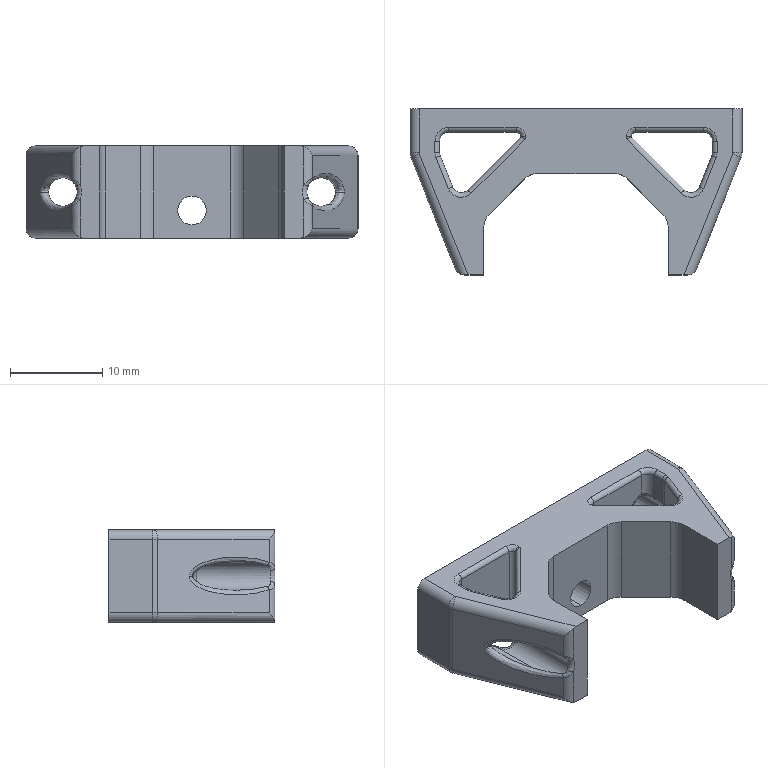Part | SolidWorks | features Fillet 4, Extrusion 1, ICE 1 | 1 solid | 138 faces | box 36 x 18 x 10 mm | volume 2888 mm3 | cylinder 62 | plane 28 | torus 26 | spline 22 | commonest cylinder face diameters 1 x26 2 x22 3.1 x8 4 x4 3 x2